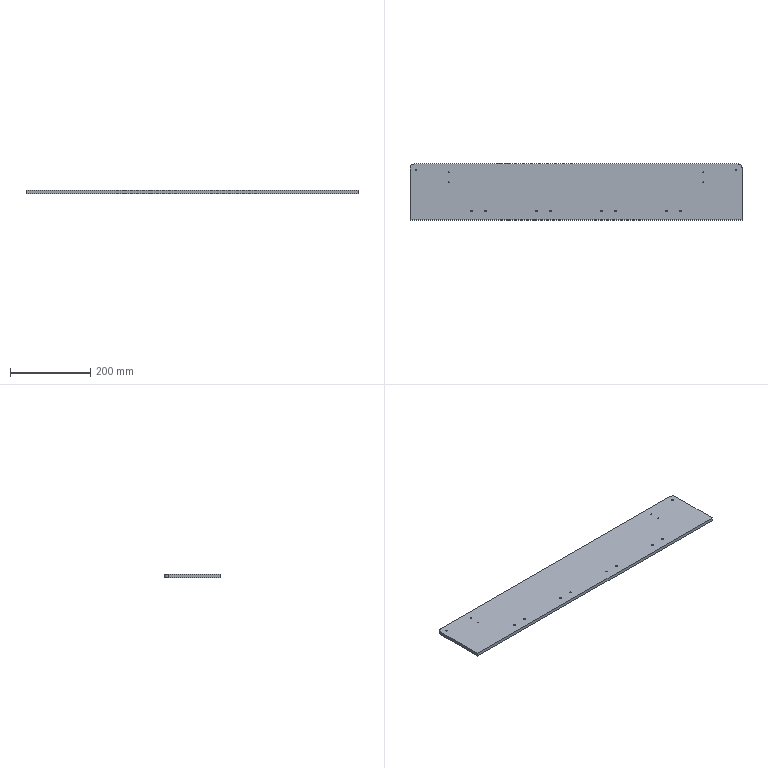Part | NX | 1 solid | 22 faces | box 830 x 140 x 8 mm | volume 927991 mm3 | cylinder 16 | plane 6 | commonest cylinder face diameters 4.2 x10 2.5 x4 20 x2
STEP:
#1=CARTESIAN_POINT('',(-415.,60.,0.));
#2=VERTEX_POINT('',#1);
#3=CARTESIAN_POINT('',(-415.,-70.,0.));
#4=VERTEX_POINT('',#3);
#5=CARTESIAN_POINT('',(-415.,70.,0.));
#6=DIRECTION('',(0.,-1.,0.));
#7=VECTOR('',#6,1000.);
#8=LINE('',#5,#7);
#9=EDGE_CURVE('',#2,#4,#8,.T.);
#10=ORIENTED_EDGE('',*,*,#9,.F.);
#11=CARTESIAN_POINT('',(-415.,60.,-8.));
#12=VERTEX_POINT('',#11);
#13=CARTESIAN_POINT('',(-415.,60.,-8.));
#14=DIRECTION('',(0.,0.,1.));
#15=VECTOR('',#14,1000.);
#16=LINE('',#13,#15);
#17=EDGE_CURVE('',#2,#12,#16,.F.);
#18=ORIENTED_EDGE('',*,*,#17,.T.);
#19=CARTESIAN_POINT('',(-415.,-70.,-8.));
#20=VERTEX_POINT('',#19);
#21=CARTESIAN_POINT('',(-415.,70.,-8.));
#22=DIRECTION('',(0.,-1.,0.));
#23=VECTOR('',#22,1000.);
#24=LINE('',#21,#23);
#25=EDGE_CURVE('',#12,#20,#24,.T.);
#26=ORIENTED_EDGE('',*,*,#25,.T.);
#27=CARTESIAN_POINT('',(-415.,-70.,-8.));
#28=DIRECTION('',(0.,0.,1.));
#29=VECTOR('',#28,1000.);
#30=LINE('',#27,#29);
#31=EDGE_CURVE('',#20,#4,#30,.T.);
#32=ORIENTED_EDGE('',*,*,#31,.T.);
#33=EDGE_LOOP('',(#10,#18,#26,#32));
#34=FACE_BOUND('',#33,.T.);
#35=CARTESIAN_POINT('',(-415.,70.,-8.));
#36=DIRECTION('',(-1.,0.,0.));
#37=DIRECTION('',(0.,-1.,0.));
#38=AXIS2_PLACEMENT_3D('',#35,#36,#37);
#39=PLANE('',#38);
#40=ADVANCED_FACE('',(#34),#39,.T.);
#41=CARTESIAN_POINT('',(405.,70.,0.));
#42=VERTEX_POINT('',#41);
#43=CARTESIAN_POINT('',(-405.,70.,0.));
#44=VERTEX_POINT('',#43);
#45=CARTESIAN_POINT('',(415.,70.,0.));
#46=DIRECTION('',(-1.,0.,0.));
#47=VECTOR('',#46,1000.);
#48=LINE('',#45,#47);
#49=EDGE_CURVE('',#42,#44,#48,.T.);
#50=ORIENTED_EDGE('',*,*,#49,.F.);
#51=CARTESIAN_POINT('',(405.,70.,-8.));
#52=VERTEX_POINT('',#51);
#53=CARTESIAN_POINT('',(405.,70.,-8.));
#54=DIRECTION('',(0.,0.,1.));
#55=VECTOR('',#54,1000.);
#56=LINE('',#53,#55);
#57=EDGE_CURVE('',#42,#52,#56,.F.);
#58=ORIENTED_EDGE('',*,*,#57,.T.);
#59=CARTESIAN_POINT('',(-405.,70.,-8.));
#60=VERTEX_POINT('',#59);
#61=CARTESIAN_POINT('',(415.,70.,-8.));
#62=DIRECTION('',(-1.,0.,0.));
#63=VECTOR('',#62,1000.);
#64=LINE('',#61,#63);
#65=EDGE_CURVE('',#52,#60,#64,.T.);
#66=ORIENTED_EDGE('',*,*,#65,.T.);
#67=CARTESIAN_POINT('',(-405.,70.,-8.));
#68=DIRECTION('',(0.,0.,1.));
#69=VECTOR('',#68,1000.);
#70=LINE('',#67,#69);
#71=EDGE_CURVE('',#60,#44,#70,.T.);
#72=ORIENTED_EDGE('',*,*,#71,.T.);
#73=EDGE_LOOP('',(#50,#58,#66,#72));
#74=FACE_BOUND('',#73,.T.);
#75=CARTESIAN_POINT('',(415.,70.,-8.));
#76=DIRECTION('',(0.,1.,0.));
#77=DIRECTION('',(-1.,0.,0.));
#78=AXIS2_PLACEMENT_3D('',#75,#76,#77);
#79=PLANE('',#78);
#80=ADVANCED_FACE('',(#74),#79,.T.);
#81=CARTESIAN_POINT('',(415.,-70.,-8.));
#82=VERTEX_POINT('',#81);
#83=CARTESIAN_POINT('',(415.,60.,-8.));
#84=VERTEX_POINT('',#83);
#85=CARTESIAN_POINT('',(415.,70.,-8.));
#86=DIRECTION('',(0.,1.,0.));
#87=VECTOR('',#86,1000.);
#88=LINE('',#85,#87);
#89=EDGE_CURVE('',#82,#84,#88,.T.);
#90=ORIENTED_EDGE('',*,*,#89,.T.);
#91=CARTESIAN_POINT('',(415.,60.,0.));
#92=VERTEX_POINT('',#91);
#93=CARTESIAN_POINT('',(415.,60.,-8.));
#94=DIRECTION('',(0.,0.,1.));
#95=VECTOR('',#94,1000.);
#96=LINE('',#93,#95);
#97=EDGE_CURVE('',#84,#92,#96,.T.);
#98=ORIENTED_EDGE('',*,*,#97,.T.);
#99=CARTESIAN_POINT('',(415.,-70.,0.));
#100=VERTEX_POINT('',#99);
#101=CARTESIAN_POINT('',(415.,70.,0.));
#102=DIRECTION('',(0.,1.,0.));
#103=VECTOR('',#102,1000.);
#104=LINE('',#101,#103);
#105=EDGE_CURVE('',#100,#92,#104,.T.);
#106=ORIENTED_EDGE('',*,*,#105,.F.);
#107=CARTESIAN_POINT('',(415.,-70.,-8.));
#108=DIRECTION('',(0.,0.,1.));
#109=VECTOR('',#108,1000.);
#110=LINE('',#107,#109);
#111=EDGE_CURVE('',#82,#100,#110,.T.);
#112=ORIENTED_EDGE('',*,*,#111,.F.);
#113=EDGE_LOOP('',(#90,#98,#106,#112));
#114=FACE_BOUND('',#113,.T.);
#115=CARTESIAN_POINT('',(415.,70.,-8.));
#116=DIRECTION('',(1.,0.,0.));
#117=DIRECTION('',(0.,0.,-1.));
#118=AXIS2_PLACEMENT_3D('',#115,#116,#117);
#119=PLANE('',#118);
#120=ADVANCED_FACE('',(#114),#119,.T.);
#121=CARTESIAN_POINT('',(415.,-70.,0.));
#122=DIRECTION('',(1.,0.,0.));
#123=VECTOR('',#122,1000.);
#124=LINE('',#121,#123);
#125=EDGE_CURVE('',#4,#100,#124,.T.);
#126=ORIENTED_EDGE('',*,*,#125,.F.);
#127=ORIENTED_EDGE('',*,*,#31,.F.);
#128=CARTESIAN_POINT('',(415.,-70.,-8.));
#129=DIRECTION('',(1.,0.,0.));
#130=VECTOR('',#129,1000.);
#131=LINE('',#128,#130);
#132=EDGE_CURVE('',#20,#82,#131,.T.);
#133=ORIENTED_EDGE('',*,*,#132,.T.);
#134=ORIENTED_EDGE('',*,*,#111,.T.);
#135=EDGE_LOOP('',(#126,#127,#133,#134));
#136=FACE_BOUND('',#135,.T.);
#137=CARTESIAN_POINT('',(415.,-70.,-8.));
#138=DIRECTION('',(0.,-1.,0.));
#139=DIRECTION('',(1.,0.,0.));
#140=AXIS2_PLACEMENT_3D('',#137,#138,#139);
#141=PLANE('',#140);
#142=ADVANCED_FACE('',(#136),#141,.T.);
#143=CARTESIAN_POINT('',(397.9,55.,-8.));
#144=VERTEX_POINT('',#143);
#145=CARTESIAN_POINT('',(400.,55.,-8.));
#146=DIRECTION('',(0.,0.,-1.));
#147=DIRECTION('',(-1.,0.,0.));
#148=AXIS2_PLACEMENT_3D('',#145,#146,#147);
#149=CIRCLE('',#148,2.1);
#150=EDGE_CURVE('',#144,#144,#149,.T.);
#151=ORIENTED_EDGE('',*,*,#150,.F.);
#152=EDGE_LOOP('',(#151));
#153=FACE_BOUND('',#152,.T.);
#154=CARTESIAN_POINT('',(-402.1,55.,-8.));
#155=VERTEX_POINT('',#154);
#156=CARTESIAN_POINT('',(-400.,55.,-8.));
#157=DIRECTION('',(0.,0.,-1.));
#158=DIRECTION('',(-1.,0.,0.));
#159=AXIS2_PLACEMENT_3D('',#156,#157,#158);
#160=CIRCLE('',#159,2.1);
#161=EDGE_CURVE('',#155,#155,#160,.T.);
#162=ORIENTED_EDGE('',*,*,#161,.F.);
#163=EDGE_LOOP('',(#162));
#164=FACE_BOUND('',#163,.T.);
#165=CARTESIAN_POINT('',(-229.1,-47.5,-8.));
#166=VERTEX_POINT('',#165);
#167=CARTESIAN_POINT('',(-227.,-47.5,-8.));
#168=DIRECTION('',(0.,0.,-1.));
#169=DIRECTION('',(-1.,0.,0.));
#170=AXIS2_PLACEMENT_3D('',#167,#168,#169);
#171=CIRCLE('',#170,2.1);
#172=EDGE_CURVE('',#166,#166,#171,.T.);
#173=ORIENTED_EDGE('',*,*,#172,.F.);
#174=EDGE_LOOP('',(#173));
#175=FACE_BOUND('',#174,.T.);
#176=CARTESIAN_POINT('',(-264.1,-47.5,-8.));
#177=VERTEX_POINT('',#176);
#178=CARTESIAN_POINT('',(-262.,-47.5,-8.));
#179=DIRECTION('',(0.,0.,-1.));
#180=DIRECTION('',(-1.,0.,0.));
#181=AXIS2_PLACEMENT_3D('',#178,#179,#180);
#182=CIRCLE('',#181,2.1);
#183=EDGE_CURVE('',#177,#177,#182,.T.);
#184=ORIENTED_EDGE('',*,*,#183,.F.);
#185=EDGE_LOOP('',(#184));
#186=FACE_BOUND('',#185,.T.);
#187=CARTESIAN_POINT('',(-66.1,-47.5,-8.));
#188=VERTEX_POINT('',#187);
#189=CARTESIAN_POINT('',(-64.,-47.5,-8.));
#190=DIRECTION('',(0.,0.,-1.));
#191=DIRECTION('',(-1.,0.,0.));
#192=AXIS2_PLACEMENT_3D('',#189,#190,#191);
#193=CIRCLE('',#192,2.1);
#194=EDGE_CURVE('',#188,#188,#193,.T.);
#195=ORIENTED_EDGE('',*,*,#194,.F.);
#196=EDGE_LOOP('',(#195));
#197=FACE_BOUND('',#196,.T.);
#198=CARTESIAN_POINT('',(-101.1,-47.5,-8.));
#199=VERTEX_POINT('',#198);
#200=CARTESIAN_POINT('',(-99.,-47.5,-8.));
#201=DIRECTION('',(0.,0.,-1.));
#202=DIRECTION('',(-1.,0.,0.));
#203=AXIS2_PLACEMENT_3D('',#200,#201,#202);
#204=CIRCLE('',#203,2.1);
#205=EDGE_CURVE('',#199,#199,#204,.T.);
#206=ORIENTED_EDGE('',*,*,#205,.F.);
#207=EDGE_LOOP('',(#206));
#208=FACE_BOUND('',#207,.T.);
#209=CARTESIAN_POINT('',(96.9,-47.5,-8.));
#210=VERTEX_POINT('',#209);
#211=CARTESIAN_POINT('',(99.,-47.5,-8.));
#212=DIRECTION('',(0.,0.,-1.));
#213=DIRECTION('',(-1.,0.,0.));
#214=AXIS2_PLACEMENT_3D('',#211,#212,#213);
#215=CIRCLE('',#214,2.1);
#216=EDGE_CURVE('',#210,#210,#215,.T.);
#217=ORIENTED_EDGE('',*,*,#216,.F.);
#218=EDGE_LOOP('',(#217));
#219=FACE_BOUND('',#218,.T.);
#220=CARTESIAN_POINT('',(61.9,-47.5,-8.));
#221=VERTEX_POINT('',#220);
#222=CARTESIAN_POINT('',(64.,-47.5,-8.));
#223=DIRECTION('',(0.,0.,-1.));
#224=DIRECTION('',(-1.,0.,0.));
#225=AXIS2_PLACEMENT_3D('',#222,#223,#224);
#226=CIRCLE('',#225,2.1);
#227=EDGE_CURVE('',#221,#221,#226,.T.);
#228=ORIENTED_EDGE('',*,*,#227,.F.);
#229=EDGE_LOOP('',(#228));
#230=FACE_BOUND('',#229,.T.);
#231=CARTESIAN_POINT('',(259.9,-47.5,-8.));
#232=VERTEX_POINT('',#231);
#233=CARTESIAN_POINT('',(262.,-47.5,-8.));
#234=DIRECTION('',(0.,0.,-1.));
#235=DIRECTION('',(-1.,0.,0.));
#236=AXIS2_PLACEMENT_3D('',#233,#234,#235);
#237=CIRCLE('',#236,2.1);
#238=EDGE_CURVE('',#232,#232,#237,.T.);
#239=ORIENTED_EDGE('',*,*,#238,.F.);
#240=EDGE_LOOP('',(#239));
#241=FACE_BOUND('',#240,.T.);
#242=CARTESIAN_POINT('',(224.9,-47.5,-8.));
#243=VERTEX_POINT('',#242);
#244=CARTESIAN_POINT('',(227.,-47.5,-8.));
#245=DIRECTION('',(0.,0.,-1.));
#246=DIRECTION('',(-1.,0.,0.));
#247=AXIS2_PLACEMENT_3D('',#244,#245,#246);
#248=CIRCLE('',#247,2.1);
#249=EDGE_CURVE('',#243,#243,#248,.T.);
#250=ORIENTED_EDGE('',*,*,#249,.F.);
#251=EDGE_LOOP('',(#250));
#252=FACE_BOUND('',#251,.T.);
#253=CARTESIAN_POINT('',(-319.75,49.,-8.));
#254=VERTEX_POINT('',#253);
#255=CARTESIAN_POINT('',(-318.5,49.,-8.));
#256=DIRECTION('',(0.,0.,-1.));
#257=DIRECTION('',(-1.,0.,0.));
#258=AXIS2_PLACEMENT_3D('',#255,#256,#257);
#259=CIRCLE('',#258,1.25);
#260=EDGE_CURVE('',#254,#254,#259,.T.);
#261=ORIENTED_EDGE('',*,*,#260,.F.);
#262=EDGE_LOOP('',(#261));
#263=FACE_BOUND('',#262,.T.);
#264=CARTESIAN_POINT('',(-319.75,24.,-8.));
#265=VERTEX_POINT('',#264);
#266=CARTESIAN_POINT('',(-318.5,24.,-8.));
#267=DIRECTION('',(0.,0.,-1.));
#268=DIRECTION('',(-1.,0.,0.));
#269=AXIS2_PLACEMENT_3D('',#266,#267,#268);
#270=CIRCLE('',#269,1.25);
#271=EDGE_CURVE('',#265,#265,#270,.T.);
#272=ORIENTED_EDGE('',*,*,#271,.F.);
#273=EDGE_LOOP('',(#272));
#274=FACE_BOUND('',#273,.T.);
#275=CARTESIAN_POINT('',(317.25,24.,-8.));
#276=VERTEX_POINT('',#275);
#277=CARTESIAN_POINT('',(318.5,24.,-8.));
#278=DIRECTION('',(0.,0.,-1.));
#279=DIRECTION('',(-1.,0.,0.));
#280=AXIS2_PLACEMENT_3D('',#277,#278,#279);
#281=CIRCLE('',#280,1.25);
#282=EDGE_CURVE('',#276,#276,#281,.T.);
#283=ORIENTED_EDGE('',*,*,#282,.F.);
#284=EDGE_LOOP('',(#283));
#285=FACE_BOUND('',#284,.T.);
#286=CARTESIAN_POINT('',(317.25,49.,-8.));
#287=VERTEX_POINT('',#286);
#288=CARTESIAN_POINT('',(318.5,49.,-8.));
#289=DIRECTION('',(0.,0.,-1.));
#290=DIRECTION('',(-1.,0.,0.));
#291=AXIS2_PLACEMENT_3D('',#288,#289,#290);
#292=CIRCLE('',#291,1.25);
#293=EDGE_CURVE('',#287,#287,#292,.T.);
#294=ORIENTED_EDGE('',*,*,#293,.F.);
#295=EDGE_LOOP('',(#294));
#296=FACE_BOUND('',#295,.T.);
#297=ORIENTED_EDGE('',*,*,#65,.F.);
#298=CARTESIAN_POINT('',(405.,60.,-8.));
#299=DIRECTION('',(0.,0.,-1.));
#300=DIRECTION('',(-1.,0.,0.));
#301=AXIS2_PLACEMENT_3D('',#298,#299,#300);
#302=CIRCLE('',#301,10.);
#303=EDGE_CURVE('',#52,#84,#302,.T.);
#304=ORIENTED_EDGE('',*,*,#303,.T.);
#305=ORIENTED_EDGE('',*,*,#89,.F.);
#306=ORIENTED_EDGE('',*,*,#132,.F.);
#307=ORIENTED_EDGE('',*,*,#25,.F.);
#308=CARTESIAN_POINT('',(-405.,60.,-8.));
#309=DIRECTION('',(0.,0.,-1.));
#310=DIRECTION('',(-1.,0.,0.));
#311=AXIS2_PLACEMENT_3D('',#308,#309,#310);
#312=CIRCLE('',#311,10.);
#313=EDGE_CURVE('',#12,#60,#312,.T.);
#314=ORIENTED_EDGE('',*,*,#313,.T.);
#315=EDGE_LOOP('',(#297,#304,#305,#306,#307,#314));
#316=FACE_BOUND('',#315,.T.);
#317=CARTESIAN_POINT('',(0.,0.,-8.));
#318=DIRECTION('',(0.,0.,-1.));
#319=DIRECTION('',(-1.,0.,0.));
#320=AXIS2_PLACEMENT_3D('',#317,#318,#319);
#321=PLANE('',#320);
#322=ADVANCED_FACE('',(#153,#164,#175,#186,#197,#208,#219,#230,#241,#252,#263,#274,#285,#296,#316),#321,.T.);
#323=CARTESIAN_POINT('',(397.9,55.,0.));
#324=VERTEX_POINT('',#323);
#325=CARTESIAN_POINT('',(400.,55.,0.));
#326=DIRECTION('',(0.,0.,-1.));
#327=DIRECTION('',(-1.,0.,0.));
#328=AXIS2_PLACEMENT_3D('',#325,#326,#327);
#329=CIRCLE('',#328,2.1);
#330=EDGE_CURVE('',#324,#324,#329,.T.);
#331=ORIENTED_EDGE('',*,*,#330,.T.);
#332=EDGE_LOOP('',(#331));
#333=FACE_BOUND('',#332,.T.);
#334=CARTESIAN_POINT('',(-402.1,55.,0.));
#335=VERTEX_POINT('',#334);
#336=CARTESIAN_POINT('',(-400.,55.,0.));
#337=DIRECTION('',(0.,0.,-1.));
#338=DIRECTION('',(-1.,0.,0.));
#339=AXIS2_PLACEMENT_3D('',#336,#337,#338);
#340=CIRCLE('',#339,2.1);
#341=EDGE_CURVE('',#335,#335,#340,.T.);
#342=ORIENTED_EDGE('',*,*,#341,.T.);
#343=EDGE_LOOP('',(#342));
#344=FACE_BOUND('',#343,.T.);
#345=CARTESIAN_POINT('',(-229.1,-47.5,0.));
#346=VERTEX_POINT('',#345);
#347=CARTESIAN_POINT('',(-227.,-47.5,0.));
#348=DIRECTION('',(0.,0.,-1.));
#349=DIRECTION('',(-1.,0.,0.));
#350=AXIS2_PLACEMENT_3D('',#347,#348,#349);
#351=CIRCLE('',#350,2.1);
#352=EDGE_CURVE('',#346,#346,#351,.T.);
#353=ORIENTED_EDGE('',*,*,#352,.T.);
#354=EDGE_LOOP('',(#353));
#355=FACE_BOUND('',#354,.T.);
#356=CARTESIAN_POINT('',(-264.1,-47.5,0.));
#357=VERTEX_POINT('',#356);
#358=CARTESIAN_POINT('',(-262.,-47.5,0.));
#359=DIRECTION('',(0.,0.,-1.));
#360=DIRECTION('',(-1.,0.,0.));
#361=AXIS2_PLACEMENT_3D('',#358,#359,#360);
#362=CIRCLE('',#361,2.1);
#363=EDGE_CURVE('',#357,#357,#362,.T.);
#364=ORIENTED_EDGE('',*,*,#363,.T.);
#365=EDGE_LOOP('',(#364));
#366=FACE_BOUND('',#365,.T.);
#367=CARTESIAN_POINT('',(-66.1,-47.5,0.));
#368=VERTEX_POINT('',#367);
#369=CARTESIAN_POINT('',(-64.,-47.5,0.));
#370=DIRECTION('',(0.,0.,-1.));
#371=DIRECTION('',(-1.,0.,0.));
#372=AXIS2_PLACEMENT_3D('',#369,#370,#371);
#373=CIRCLE('',#372,2.1);
#374=EDGE_CURVE('',#368,#368,#373,.T.);
#375=ORIENTED_EDGE('',*,*,#374,.T.);
#376=EDGE_LOOP('',(#375));
#377=FACE_BOUND('',#376,.T.);
#378=CARTESIAN_POINT('',(-101.1,-47.5,0.));
#379=VERTEX_POINT('',#378);
#380=CARTESIAN_POINT('',(-99.,-47.5,0.));
#381=DIRECTION('',(0.,0.,-1.));
#382=DIRECTION('',(-1.,0.,0.));
#383=AXIS2_PLACEMENT_3D('',#380,#381,#382);
#384=CIRCLE('',#383,2.1);
#385=EDGE_CURVE('',#379,#379,#384,.T.);
#386=ORIENTED_EDGE('',*,*,#385,.T.);
#387=EDGE_LOOP('',(#386));
#388=FACE_BOUND('',#387,.T.);
#389=CARTESIAN_POINT('',(96.9,-47.5,0.));
#390=VERTEX_POINT('',#389);
#391=CARTESIAN_POINT('',(99.,-47.5,0.));
#392=DIRECTION('',(0.,0.,-1.));
#393=DIRECTION('',(-1.,0.,0.));
#394=AXIS2_PLACEMENT_3D('',#391,#392,#393);
#395=CIRCLE('',#394,2.1);
#396=EDGE_CURVE('',#390,#390,#395,.T.);
#397=ORIENTED_EDGE('',*,*,#396,.T.);
#398=EDGE_LOOP('',(#397));
#399=FACE_BOUND('',#398,.T.);
#400=CARTESIAN_POINT('',(61.9,-47.5,0.));
#401=VERTEX_POINT('',#400);
#402=CARTESIAN_POINT('',(64.,-47.5,0.));
#403=DIRECTION('',(0.,0.,-1.));
#404=DIRECTION('',(-1.,0.,0.));
#405=AXIS2_PLACEMENT_3D('',#402,#403,#404);
#406=CIRCLE('',#405,2.1);
#407=EDGE_CURVE('',#401,#401,#406,.T.);
#408=ORIENTED_EDGE('',*,*,#407,.T.);
#409=EDGE_LOOP('',(#408));
#410=FACE_BOUND('',#409,.T.);
#411=CARTESIAN_POINT('',(259.9,-47.5,0.));
#412=VERTEX_POINT('',#411);
#413=CARTESIAN_POINT('',(262.,-47.5,0.));
#414=DIRECTION('',(0.,0.,-1.));
#415=DIRECTION('',(-1.,0.,0.));
#416=AXIS2_PLACEMENT_3D('',#413,#414,#415);
#417=CIRCLE('',#416,2.1);
#418=EDGE_CURVE('',#412,#412,#417,.T.);
#419=ORIENTED_EDGE('',*,*,#418,.T.);
#420=EDGE_LOOP('',(#419));
#421=FACE_BOUND('',#420,.T.);
#422=CARTESIAN_POINT('',(224.9,-47.5,0.));
#423=VERTEX_POINT('',#422);
#424=CARTESIAN_POINT('',(227.,-47.5,0.));
#425=DIRECTION('',(0.,0.,-1.));
#426=DIRECTION('',(-1.,0.,0.));
#427=AXIS2_PLACEMENT_3D('',#424,#425,#426);
#428=CIRCLE('',#427,2.1);
#429=EDGE_CURVE('',#423,#423,#428,.T.);
#430=ORIENTED_EDGE('',*,*,#429,.T.);
#431=EDGE_LOOP('',(#430));
#432=FACE_BOUND('',#431,.T.);
#433=CARTESIAN_POINT('',(-319.75,49.,0.));
#434=VERTEX_POINT('',#433);
#435=CARTESIAN_POINT('',(-318.5,49.,0.));
#436=DIRECTION('',(0.,0.,-1.));
#437=DIRECTION('',(-1.,0.,0.));
#438=AXIS2_PLACEMENT_3D('',#435,#436,#437);
#439=CIRCLE('',#438,1.25);
#440=EDGE_CURVE('',#434,#434,#439,.T.);
#441=ORIENTED_EDGE('',*,*,#440,.T.);
#442=EDGE_LOOP('',(#441));
#443=FACE_BOUND('',#442,.T.);
#444=CARTESIAN_POINT('',(-319.75,24.,0.));
#445=VERTEX_POINT('',#444);
#446=CARTESIAN_POINT('',(-318.5,24.,0.));
#447=DIRECTION('',(0.,0.,-1.));
#448=DIRECTION('',(-1.,0.,0.));
#449=AXIS2_PLACEMENT_3D('',#446,#447,#448);
#450=CIRCLE('',#449,1.25);
#451=EDGE_CURVE('',#445,#445,#450,.T.);
#452=ORIENTED_EDGE('',*,*,#451,.T.);
#453=EDGE_LOOP('',(#452));
#454=FACE_BOUND('',#453,.T.);
#455=CARTESIAN_POINT('',(317.25,24.,0.));
#456=VERTEX_POINT('',#455);
#457=CARTESIAN_POINT('',(318.5,24.,0.));
#458=DIRECTION('',(0.,0.,-1.));
#459=DIRECTION('',(-1.,0.,0.));
#460=AXIS2_PLACEMENT_3D('',#457,#458,#459);
#461=CIRCLE('',#460,1.25);
#462=EDGE_CURVE('',#456,#456,#461,.T.);
#463=ORIENTED_EDGE('',*,*,#462,.T.);
#464=EDGE_LOOP('',(#463));
#465=FACE_BOUND('',#464,.T.);
#466=CARTESIAN_POINT('',(317.25,49.,0.));
#467=VERTEX_POINT('',#466);
#468=CARTESIAN_POINT('',(318.5,49.,0.));
#469=DIRECTION('',(0.,0.,-1.));
#470=DIRECTION('',(-1.,0.,0.));
#471=AXIS2_PLACEMENT_3D('',#468,#469,#470);
#472=CIRCLE('',#471,1.25);
#473=EDGE_CURVE('',#467,#467,#472,.T.);
#474=ORIENTED_EDGE('',*,*,#473,.T.);
#475=EDGE_LOOP('',(#474));
#476=FACE_BOUND('',#475,.T.);
#477=ORIENTED_EDGE('',*,*,#105,.T.);
#478=CARTESIAN_POINT('',(405.,60.,0.));
#479=DIRECTION('',(0.,0.,-1.));
#480=DIRECTION('',(-1.,0.,0.));
#481=AXIS2_PLACEMENT_3D('',#478,#479,#480);
#482=CIRCLE('',#481,10.);
#483=EDGE_CURVE('',#92,#42,#482,.F.);
#484=ORIENTED_EDGE('',*,*,#483,.T.);
#485=ORIENTED_EDGE('',*,*,#49,.T.);
#486=CARTESIAN_POINT('',(-405.,60.,0.));
#487=DIRECTION('',(0.,0.,-1.));
#488=DIRECTION('',(-1.,0.,0.));
#489=AXIS2_PLACEMENT_3D('',#486,#487,#488);
#490=CIRCLE('',#489,10.);
#491=EDGE_CURVE('',#44,#2,#490,.F.);
#492=ORIENTED_EDGE('',*,*,#491,.T.);
#493=ORIENTED_EDGE('',*,*,#9,.T.);
#494=ORIENTED_EDGE('',*,*,#125,.T.);
#495=EDGE_LOOP('',(#477,#484,#485,#492,#493,#494));
#496=FACE_BOUND('',#495,.T.);
#497=CARTESIAN_POINT('',(0.,0.,0.));
#498=DIRECTION('',(0.,0.,-1.));
#499=DIRECTION('',(-1.,0.,0.));
#500=AXIS2_PLACEMENT_3D('',#497,#498,#499);
#501=PLANE('',#500);
#502=ADVANCED_FACE('',(#333,#344,#355,#366,#377,#388,#399,#410,#421,#432,#443,#454,#465,#476,#496),#501,.F.);
#503=ORIENTED_EDGE('',*,*,#473,.F.);
#504=EDGE_LOOP('',(#503));
#505=FACE_BOUND('',#504,.T.);
#506=ORIENTED_EDGE('',*,*,#293,.T.);
#507=EDGE_LOOP('',(#506));
#508=FACE_BOUND('',#507,.T.);
#509=CARTESIAN_POINT('',(318.5,49.,-8.));
#510=DIRECTION('',(0.,0.,-1.));
#511=DIRECTION('',(-1.,0.,0.));
#512=AXIS2_PLACEMENT_3D('',#509,#510,#511);
#513=CYLINDRICAL_SURFACE('',#512,1.25);
#514=ADVANCED_FACE('',(#505,#508),#513,.F.);
#515=ORIENTED_EDGE('',*,*,#462,.F.);
#516=EDGE_LOOP('',(#515));
#517=FACE_BOUND('',#516,.T.);
#518=ORIENTED_EDGE('',*,*,#282,.T.);
#519=EDGE_LOOP('',(#518));
#520=FACE_BOUND('',#519,.T.);
#521=CARTESIAN_POINT('',(318.5,24.,-8.));
#522=DIRECTION('',(0.,0.,-1.));
#523=DIRECTION('',(-1.,0.,0.));
#524=AXIS2_PLACEMENT_3D('',#521,#522,#523);
#525=CYLINDRICAL_SURFACE('',#524,1.25);
#526=ADVANCED_FACE('',(#517,#520),#525,.F.);
#527=ORIENTED_EDGE('',*,*,#451,.F.);
#528=EDGE_LOOP('',(#527));
#529=FACE_BOUND('',#528,.T.);
#530=ORIENTED_EDGE('',*,*,#271,.T.);
#531=EDGE_LOOP('',(#530));
#532=FACE_BOUND('',#531,.T.);
#533=CARTESIAN_POINT('',(-318.5,24.,-8.));
#534=DIRECTION('',(0.,0.,-1.));
#535=DIRECTION('',(-1.,0.,0.));
#536=AXIS2_PLACEMENT_3D('',#533,#534,#535);
#537=CYLINDRICAL_SURFACE('',#536,1.25);
#538=ADVANCED_FACE('',(#529,#532),#537,.F.);
#539=ORIENTED_EDGE('',*,*,#440,.F.);
#540=EDGE_LOOP('',(#539));
#541=FACE_BOUND('',#540,.T.);
#542=ORIENTED_EDGE('',*,*,#260,.T.);
#543=EDGE_LOOP('',(#542));
#544=FACE_BOUND('',#543,.T.);
#545=CARTESIAN_POINT('',(-318.5,49.,-8.));
#546=DIRECTION('',(0.,0.,-1.));
#547=DIRECTION('',(-1.,0.,0.));
#548=AXIS2_PLACEMENT_3D('',#545,#546,#547);
#549=CYLINDRICAL_SURFACE('',#548,1.25);
#550=ADVANCED_FACE('',(#541,#544),#549,.F.);
#551=ORIENTED_EDGE('',*,*,#249,.T.);
#552=EDGE_LOOP('',(#551));
#553=FACE_BOUND('',#552,.T.);
#554=ORIENTED_EDGE('',*,*,#429,.F.);
#555=EDGE_LOOP('',(#554));
#556=FACE_BOUND('',#555,.T.);
#557=CARTESIAN_POINT('',(227.,-47.5,-8.));
#558=DIRECTION('',(0.,0.,-1.));
#559=DIRECTION('',(-1.,0.,0.));
#560=AXIS2_PLACEMENT_3D('',#557,#558,#559);
#561=CYLINDRICAL_SURFACE('',#560,2.1);
#562=ADVANCED_FACE('',(#553,#556),#561,.F.);
#563=ORIENTED_EDGE('',*,*,#238,.T.);
#564=EDGE_LOOP('',(#563));
#565=FACE_BOUND('',#564,.T.);
#566=ORIENTED_EDGE('',*,*,#418,.F.);
#567=EDGE_LOOP('',(#566));
#568=FACE_BOUND('',#567,.T.);
#569=CARTESIAN_POINT('',(262.,-47.5,-8.));
#570=DIRECTION('',(0.,0.,-1.));
#571=DIRECTION('',(-1.,0.,0.));
#572=AXIS2_PLACEMENT_3D('',#569,#570,#571);
#573=CYLINDRICAL_SURFACE('',#572,2.1);
#574=ADVANCED_FACE('',(#565,#568),#573,.F.);
#575=ORIENTED_EDGE('',*,*,#227,.T.);
#576=EDGE_LOOP('',(#575));
#577=FACE_BOUND('',#576,.T.);
#578=ORIENTED_EDGE('',*,*,#407,.F.);
#579=EDGE_LOOP('',(#578));
#580=FACE_BOUND('',#579,.T.);
#581=CARTESIAN_POINT('',(64.,-47.5,-8.));
#582=DIRECTION('',(0.,0.,-1.));
#583=DIRECTION('',(-1.,0.,0.));
#584=AXIS2_PLACEMENT_3D('',#581,#582,#583);
#585=CYLINDRICAL_SURFACE('',#584,2.1);
#586=ADVANCED_FACE('',(#577,#580),#585,.F.);
#587=ORIENTED_EDGE('',*,*,#216,.T.);
#588=EDGE_LOOP('',(#587));
#589=FACE_BOUND('',#588,.T.);
#590=ORIENTED_EDGE('',*,*,#396,.F.);
#591=EDGE_LOOP('',(#590));
#592=FACE_BOUND('',#591,.T.);
#593=CARTESIAN_POINT('',(99.,-47.5,-8.));
#594=DIRECTION('',(0.,0.,-1.));
#595=DIRECTION('',(-1.,0.,0.));
#596=AXIS2_PLACEMENT_3D('',#593,#594,#595);
#597=CYLINDRICAL_SURFACE('',#596,2.1);
#598=ADVANCED_FACE('',(#589,#592),#597,.F.);
#599=ORIENTED_EDGE('',*,*,#205,.T.);
#600=EDGE_LOOP('',(#599));
#601=FACE_BOUND('',#600,.T.);
#602=ORIENTED_EDGE('',*,*,#385,.F.);
#603=EDGE_LOOP('',(#602));
#604=FACE_BOUND('',#603,.T.);
#605=CARTESIAN_POINT('',(-99.,-47.5,-8.));
#606=DIRECTION('',(0.,0.,-1.));
#607=DIRECTION('',(-1.,0.,0.));
#608=AXIS2_PLACEMENT_3D('',#605,#606,#607);
#609=CYLINDRICAL_SURFACE('',#608,2.1);
#610=ADVANCED_FACE('',(#601,#604),#609,.F.);
#611=ORIENTED_EDGE('',*,*,#194,.T.);
#612=EDGE_LOOP('',(#611));
#613=FACE_BOUND('',#612,.T.);
#614=ORIENTED_EDGE('',*,*,#374,.F.);
#615=EDGE_LOOP('',(#614));
#616=FACE_BOUND('',#615,.T.);
#617=CARTESIAN_POINT('',(-64.,-47.5,-8.));
#618=DIRECTION('',(0.,0.,-1.));
#619=DIRECTION('',(-1.,0.,0.));
#620=AXIS2_PLACEMENT_3D('',#617,#618,#619);
#621=CYLINDRICAL_SURFACE('',#620,2.1);
#622=ADVANCED_FACE('',(#613,#616),#621,.F.);
#623=ORIENTED_EDGE('',*,*,#183,.T.);
#624=EDGE_LOOP('',(#623));
#625=FACE_BOUND('',#624,.T.);
#626=ORIENTED_EDGE('',*,*,#363,.F.);
#627=EDGE_LOOP('',(#626));
#628=FACE_BOUND('',#627,.T.);
#629=CARTESIAN_POINT('',(-262.,-47.5,-8.));
#630=DIRECTION('',(0.,0.,-1.));
#631=DIRECTION('',(-1.,0.,0.));
#632=AXIS2_PLACEMENT_3D('',#629,#630,#631);
#633=CYLINDRICAL_SURFACE('',#632,2.1);
#634=ADVANCED_FACE('',(#625,#628),#633,.F.);
#635=ORIENTED_EDGE('',*,*,#172,.T.);
#636=EDGE_LOOP('',(#635));
#637=FACE_BOUND('',#636,.T.);
#638=ORIENTED_EDGE('',*,*,#352,.F.);
#639=EDGE_LOOP('',(#638));
#640=FACE_BOUND('',#639,.T.);
#641=CARTESIAN_POINT('',(-227.,-47.5,-8.));
#642=DIRECTION('',(0.,0.,-1.));
#643=DIRECTION('',(-1.,0.,0.));
#644=AXIS2_PLACEMENT_3D('',#641,#642,#643);
#645=CYLINDRICAL_SURFACE('',#644,2.1);
#646=ADVANCED_FACE('',(#637,#640),#645,.F.);
#647=ORIENTED_EDGE('',*,*,#303,.F.);
#648=ORIENTED_EDGE('',*,*,#57,.F.);
#649=ORIENTED_EDGE('',*,*,#483,.F.);
#650=ORIENTED_EDGE('',*,*,#97,.F.);
#651=EDGE_LOOP('',(#647,#648,#649,#650));
#652=FACE_BOUND('',#651,.T.);
#653=CARTESIAN_POINT('',(405.,60.,-8.));
#654=DIRECTION('',(0.,0.,1.));
#655=DIRECTION('',(1.,0.,0.));
#656=AXIS2_PLACEMENT_3D('',#653,#654,#655);
#657=CYLINDRICAL_SURFACE('',#656,10.);
#658=ADVANCED_FACE('',(#652),#657,.T.);
#659=ORIENTED_EDGE('',*,*,#313,.F.);
#660=ORIENTED_EDGE('',*,*,#17,.F.);
#661=ORIENTED_EDGE('',*,*,#491,.F.);
#662=ORIENTED_EDGE('',*,*,#71,.F.);
#663=EDGE_LOOP('',(#659,#660,#661,#662));
#664=FACE_BOUND('',#663,.T.);
#665=CARTESIAN_POINT('',(-405.,60.,-8.));
#666=DIRECTION('',(0.,0.,1.));
#667=DIRECTION('',(1.,0.,0.));
#668=AXIS2_PLACEMENT_3D('',#665,#666,#667);
#669=CYLINDRICAL_SURFACE('',#668,10.);
#670=ADVANCED_FACE('',(#664),#669,.T.);
#671=ORIENTED_EDGE('',*,*,#341,.F.);
#672=EDGE_LOOP('',(#671));
#673=FACE_BOUND('',#672,.T.);
#674=ORIENTED_EDGE('',*,*,#161,.T.);
#675=EDGE_LOOP('',(#674));
#676=FACE_BOUND('',#675,.T.);
#677=CARTESIAN_POINT('',(-400.,55.,-8.));
#678=DIRECTION('',(0.,0.,-1.));
#679=DIRECTION('',(-1.,0.,0.));
#680=AXIS2_PLACEMENT_3D('',#677,#678,#679);
#681=CYLINDRICAL_SURFACE('',#680,2.1);
#682=ADVANCED_FACE('',(#673,#676),#681,.F.);
#683=ORIENTED_EDGE('',*,*,#330,.F.);
#684=EDGE_LOOP('',(#683));
#685=FACE_BOUND('',#684,.T.);
#686=ORIENTED_EDGE('',*,*,#150,.T.);
#687=EDGE_LOOP('',(#686));
#688=FACE_BOUND('',#687,.T.);
#689=CARTESIAN_POINT('',(400.,55.,-8.));
#690=DIRECTION('',(0.,0.,-1.));
#691=DIRECTION('',(-1.,0.,0.));
#692=AXIS2_PLACEMENT_3D('',#689,#690,#691);
#693=CYLINDRICAL_SURFACE('',#692,2.1);
#694=ADVANCED_FACE('',(#685,#688),#693,.F.);
#695=CLOSED_SHELL('',(#40,#80,#120,#142,#322,#502,#514,#526,#538,#550,#562,#574,#586,#598,#610,#622,#634,#646,#658,#670,#682,#694));
#696=MANIFOLD_SOLID_BREP('',#695);
#697=(LENGTH_UNIT()NAMED_UNIT(*)SI_UNIT(.MILLI.,.METRE.));
#698=UNCERTAINTY_MEASURE_WITH_UNIT(LENGTH_MEASURE(0.00001),#697,'','');
#699=(NAMED_UNIT(*)PLANE_ANGLE_UNIT()SI_UNIT($,.RADIAN.));
#700=(NAMED_UNIT(*)SI_UNIT($,.STERADIAN.)SOLID_ANGLE_UNIT());
#701=(GEOMETRIC_REPRESENTATION_CONTEXT(3)GLOBAL_UNCERTAINTY_ASSIGNED_CONTEXT((#698))GLOBAL_UNIT_ASSIGNED_CONTEXT((#697,#699,#700))REPRESENTATION_CONTEXT('',''));
#702=ADVANCED_BREP_SHAPE_REPRESENTATION('',(#696),#701);